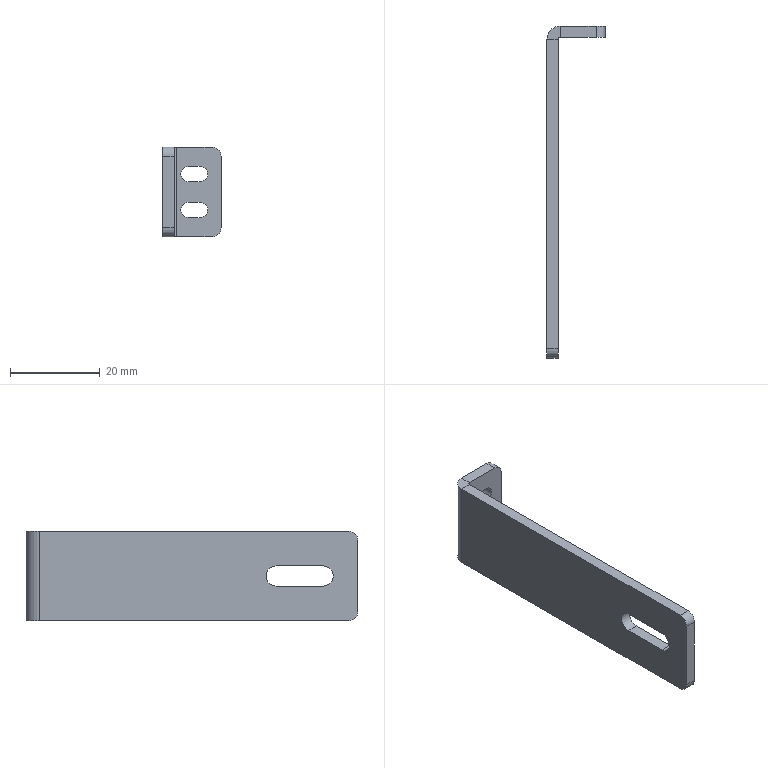Part | STEP file | 1 solid | 30 faces | box 13 x 74 x 20 mm | volume 3931 mm3 | plane 18 | cylinder 12 | commonest cylinder face diameters 3.4 x4 4 x4 4.5 x2 1 x1 6 x1